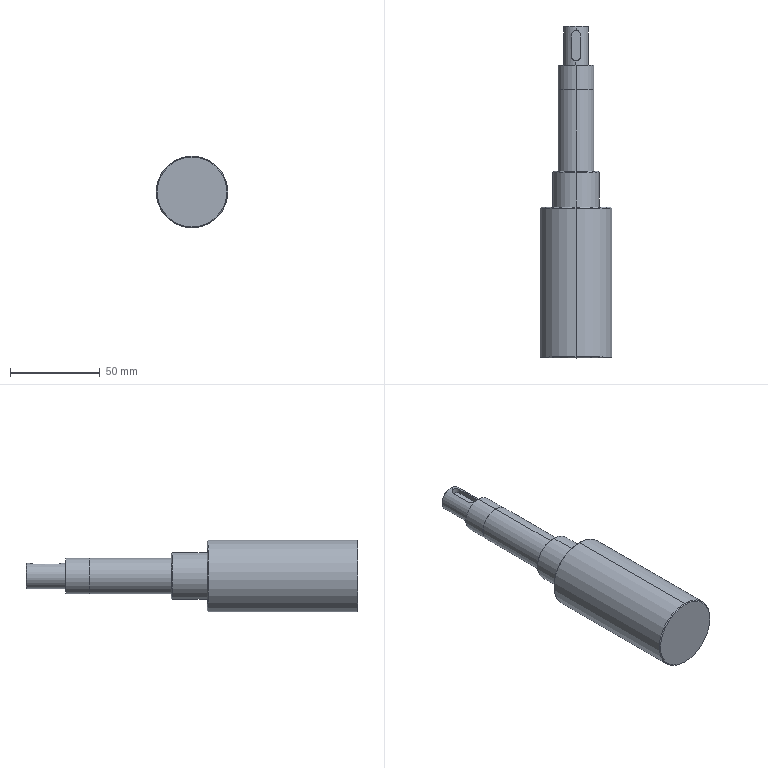Part | STEP file | ND25021-01-JDKM-02-GJ | 1 solid | 29 faces | box 40 x 185 x 40 mm | volume 137740 mm3 | cylinder 12 | plane 9 | cone 8 | commonest cylinder face diameters 5 x2 14 x2 19.8 x2 20 x2 26 x2 40 x2